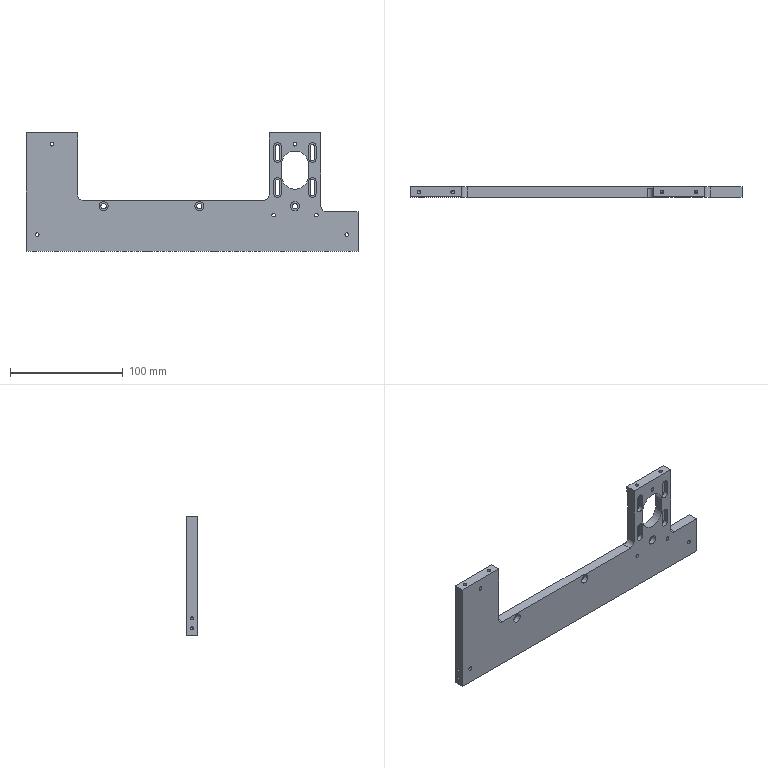CAM job | NX | 3+2 milling, drilling | part box 295 x 9 x 105 mm | stock box 300 x 12 x 110 mm
Tools:
number,name,description,diameter,corner_radius,flute_length,length,flutes
3,D3,平底铣刀-粗,3.0,0.0,20.0,75.0,2
6,D6,平底铣刀-粗,6.0,0.0,25.0,75.0,2
9,D10,平底铣刀-粗,10.0,0.0,35.0,75.0,2
18,D2-J,平底铣刀-精,2.0,0.0,50.0,75.0,2
7,D6-J,平底铣刀-精,6.0,0.0,25.0,75.0,2
1,D80R0.8飞刀,圆鼻刀-粗,80.0,0.8,50.0,75.0,2
1,D80R0.8飞刀-J,圆鼻刀-精,80.0,0.8,50.0,75.0,2
2,D6倒角刀,倒角刀,6.0,0.0,3.0,25.0,2
21,M4X0.7,丝锥,3.3,0.0,35.0,50.0,2
17,ZT4.8,钻头,4.8,0.0,35.0,50.0,2
13,钻头3.3,Twist Drill 3.3 mm,3.3,0.0,35.0,35.008,2
Operations:
program,operation,operation_type,tool,method,geometry_group,spindle_rpm,surface_speed,feed_per_tooth,feed_cut,feed_plunge,cut_length_mm,path_length_mm,cut_time_min,machine_time_min
B,动态开粗D10_COPY_1,CavityMilling,D10,动态开粗-切深K-步距K,W-B,8000.0,251.32,0.25,4000.0,100.0,43027.422,43063.222,10.757,10.76
B,底壁铣飞面精光_COPY,VolumeBased25DMillingOperation,D80R0.8飞刀-J,侧刃精光-切深K-步距G,W-B,4000.0,1005.28,0.125,1000.0,100.0,820.766,856.766,0.8208,0.8244
B,铣沉头_1,CylinderMilling,D6,METHOD,W-B,8000.0,150.796,0.125,2000.0,100.0,263.462,566.362,0.1317,0.162
B,底壁铣螺旋开粗-中_COPY,VolumeBased25DMillingOperation,D6,分层开粗-切深K-步距G,W-B,8000.0,150.796,0.075,1200.0,100.0,2026.063,2283.475,1.688,1.714
B,铣孔_1,CylinderMilling,D6-J,METHOD,W-B,8000.0,150.796,0.0375,600.0,100.0,27.906,345.506,0.0465,0.0783
B,底壁铣精光侧面-中-选底面_COPY,VolumeBased25DMillingOperation,D6-J,侧刃精光-切深K-步距G,W-B,8000.0,150.792,0.0625,1000.0,100.0,181.442,391.245,0.1814,0.2024
B,钻倒角_2,Operation,D6倒角刀,METHOD,W-B,8000.0,150.796,0.0625,1000.0,0.0,31.2,551.323,0.0312,0.0832
B,平面去毛刺6X45L_COPY,SurfaceContour,D6倒角刀,爬面_倒角-切深0-步距G,W-B,6500.0,122.519,0.1154,1500.0,100.0,1293.297,2270.778,0.8622,0.9599
A,顶面,FaceMilling,D80R0.8飞刀,侧刃精光-切深K-步距G,W-A,4000.0,1005.31,0.125,1000.0,100.0,1231.5,1267.5,1.232,1.235
A,动态开粗D10_COPY,CavityMilling,D10,动态开粗-切深K-步距K,W-A,8000.0,251.32,0.25,4000.0,100.0,29834.168,29888.568,7.458,7.464
A,底壁粗_1,VolumeBased25DMillingOperation,D10,METHOD,W-A,6000.0,113.0,0.2083,3500.0,100.0,871.8,941.505,0.2491,0.2561
A,框开粗_1,VolumeBased25DMillingOperation,D10,METHOD,W-A,6000.0,188.0,0.25,4000.0,80.0,1141.904,1190.304,0.2855,0.2903
A,打点-深0.8,Operation,D6倒角刀,NONE,W-A,8000.0,150.796,0.0312,500.0,90.0,16.2,544.914,0.0324,0.0853
A,通孔-M4螺纹底孔,Operation,钻头3.3,NONE,W-A,3000.0,31.102,0.05,300.0,90.0,94.948,668.462,0.3165,0.3738
A,通孔-5-6,Operation,ZT4.8,NONE,W-A,3000.0,45.239,0.025,150.0,90.0,39.0,290.012,0.26,0.2851
A,腰槽粗_1,VolumeBased25DMillingOperation,D3,METHOD,W-A,10000.0,62.832,0.03,600.0,100.0,5850.084,6123.792,9.75,9.777
A,底精_1,VolumeBased25DMillingOperation,D6-J,METHOD,W-A,6000.0,113.0,0.2083,1200.0,100.0,736.227,777.227,0.6135,0.6176
A,框精_1,VolumeBased25DMillingOperation,D6-J,METHOD,W-A,6000.0,113.0,0.0833,1000.0,100.0,81.453,138.253,0.0815,0.0871
A,腰槽精_1,VolumeBased25DMillingOperation,D2-J,METHOD,W-A,6000.0,37.699,0.0667,800.0,100.0,345.919,677.749,0.4324,0.4656
A,仅选体,SurfaceContour,D6倒角刀,METHOD,W-A,8000.0,150.796,0.1875,3000.0,100.0,1297.978,2022.593,0.4327,0.5051
A,钻倒角_1,Operation,D6倒角刀,METHOD,W-A,8000.0,150.796,0.0312,500.0,0.0,31.2,551.301,0.0624,0.1144
A,铣倒角_1,PlanarMilling,D6倒角刀,METHOD,W-A,8000.0,150.796,0.0312,500.0,100.0,54.061,349.837,0.1081,0.1377
A,通孔-攻牙M4,Operation,M4X0.7,METHOD,W-A,600.0,6.22,0.0006,0.7,90.0,78.0,634.566,111.429,111.484
A,底侧精_3,VolumeBased25DMillingOperation,D6-J,METHOD,W-A,6000.0,113.0,0.2083,1200.0,100.0,279.625,408.405,0.233,0.2459
A,外形半精_2,VolumeBased25DMillingOperation,D6-J,METHOD,W-A,8000.0,251.327,0.0625,1000.0,100.0,937.328,994.728,0.9373,0.9431